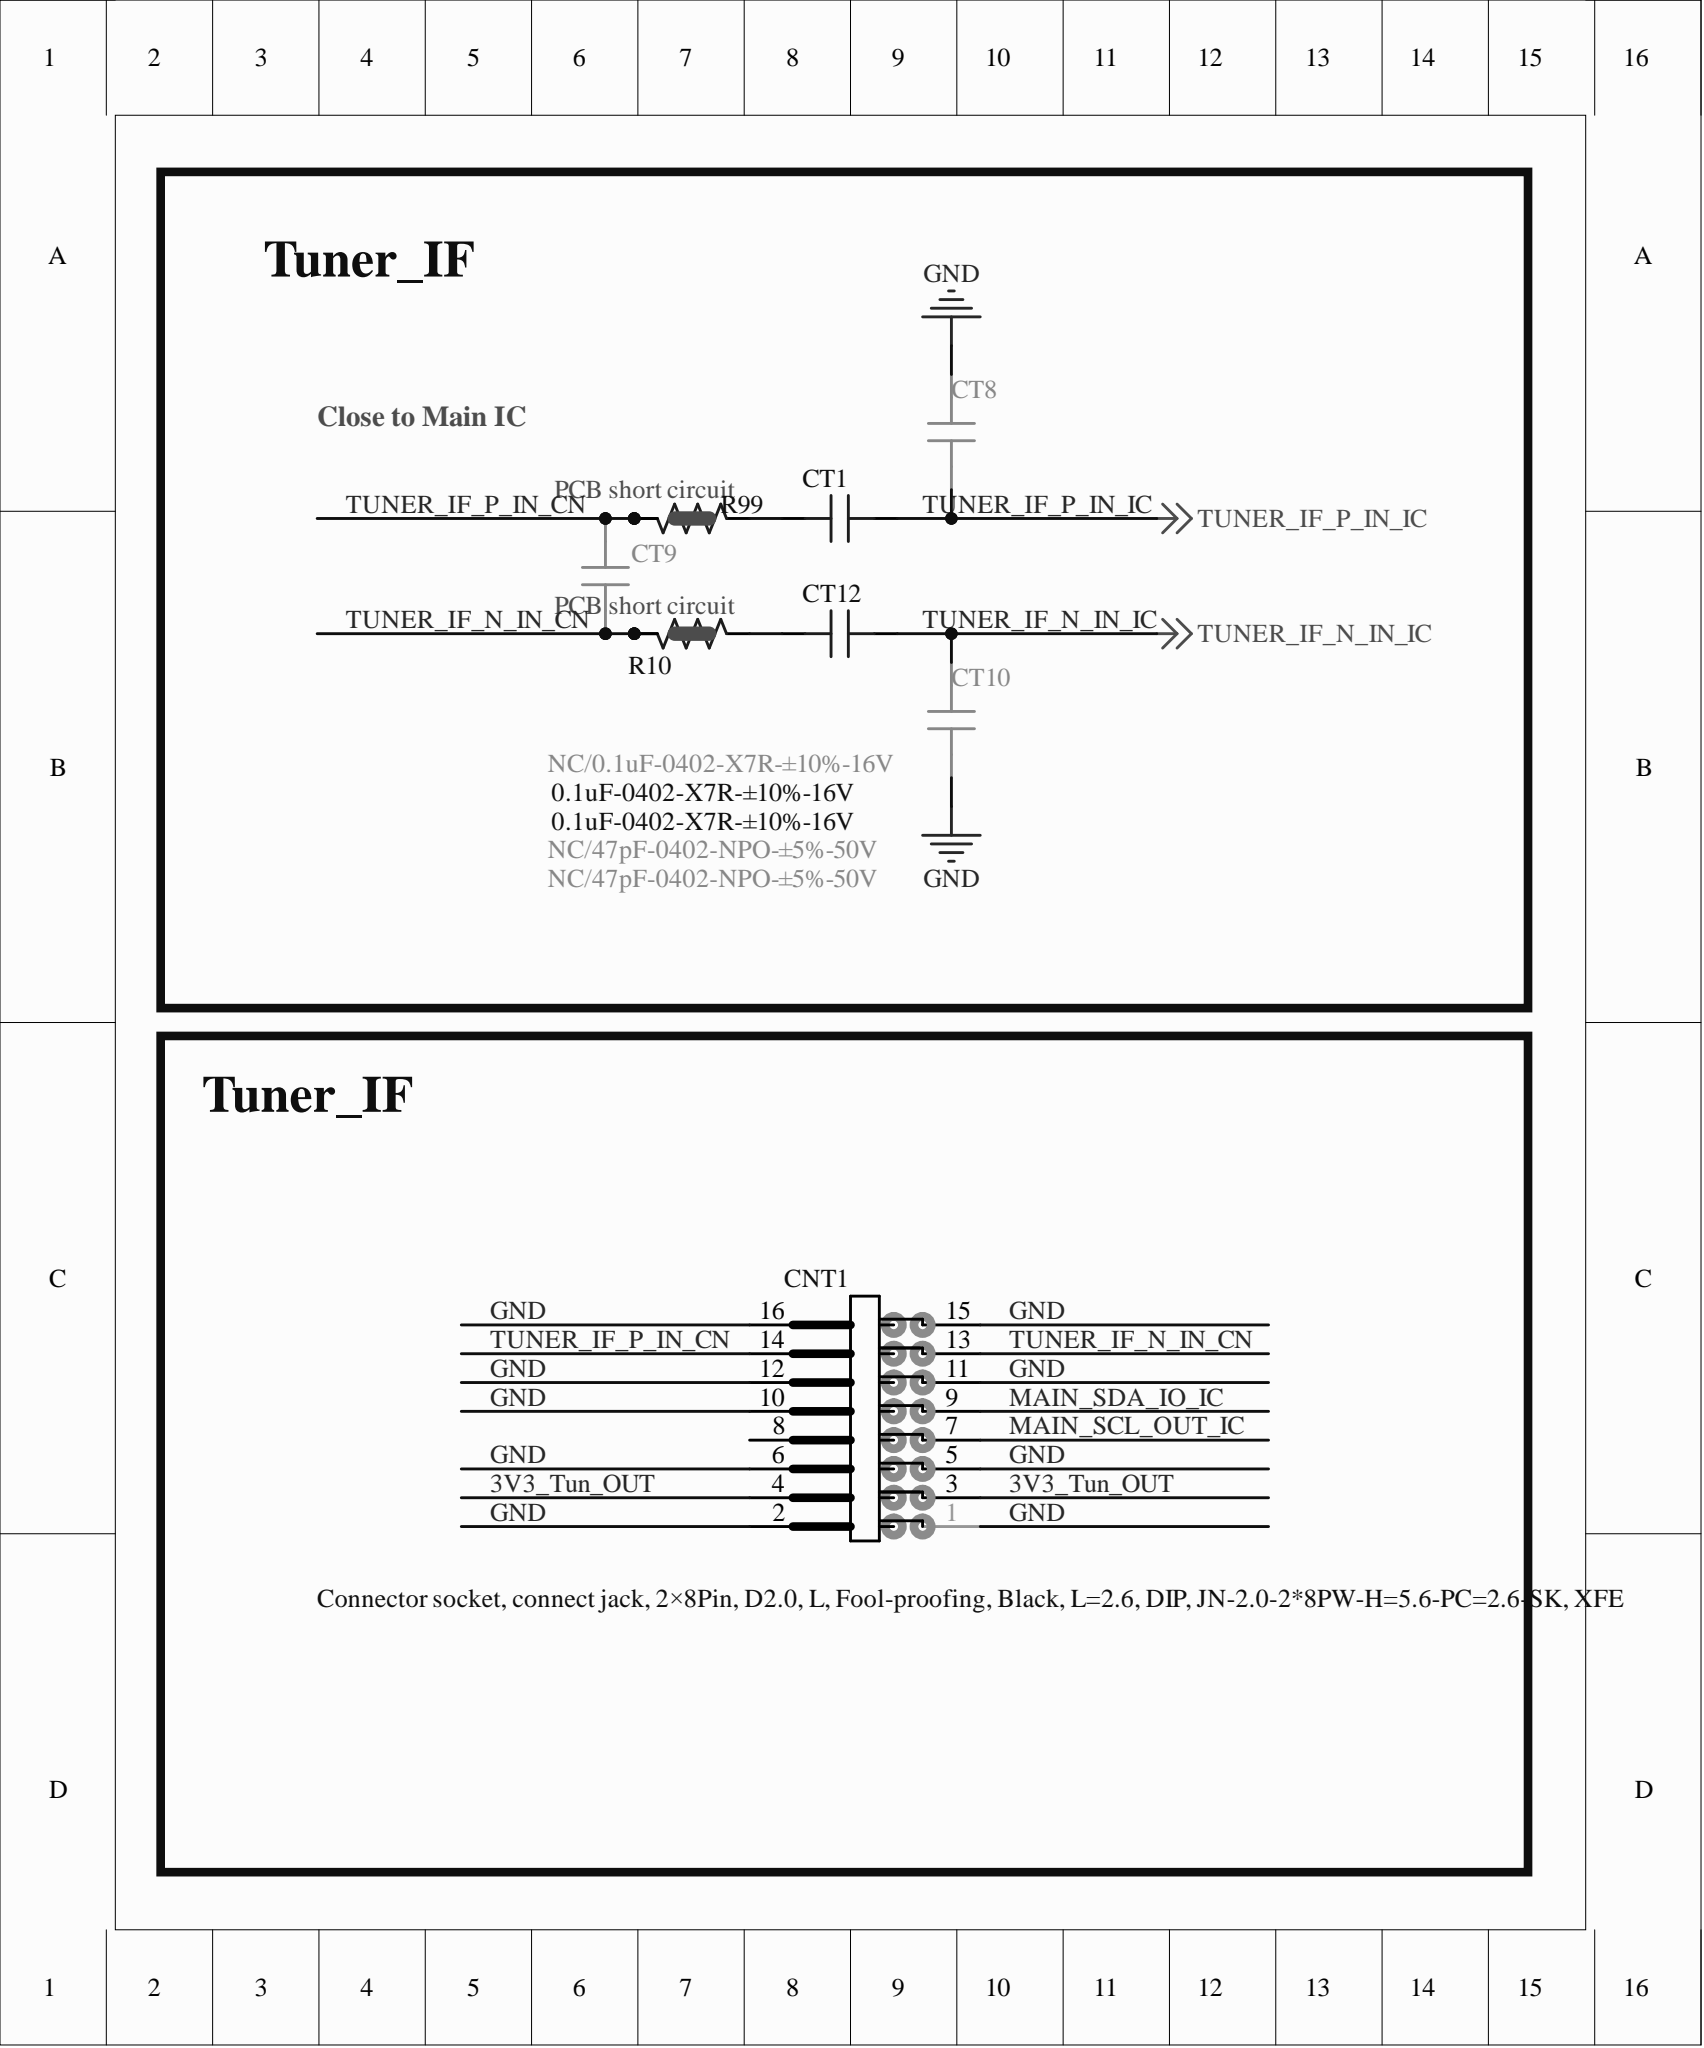Circuit board | Altium Designer | 541 parts | 263 nets | one sheet of the schematic
Parts on this sheet (reference | value | footprint):
CNT1 | Connector socket, connect jack, 2×8Pin, D2.0, L, Fool-proofing, Black, L=2.6, DIP, JN-2.0-2*8PW-H=5.6-PC=2.6-SK, XFE | SIP2*8H/2.0DM-1
CT1 | 0.1uF-0402-X7R-±10%-16V | C0402
CT8 | NC/47pF-0402-NPO-±5%-50V | C0402
CT9 | NC/0.1uF-0402-X7R-±10%-16V | C0402
CT10 | NC/47pF-0402-NPO-±5%-50V | C0402
CT12 | 0.1uF-0402-X7R-±10%-16V | C0402
R10 | NC/0ohm-0402-PCB | R0402SC
R99 | NC/0ohm-0402-PCB | R0402SC
Nets of these parts (net: part-pin ...):
TUNER_IF_P_IN_IC: CT1-1 CT8-2
TUNER_IF_P_IN_CN: CNT1-14 CT9-2 R99-2 R99-3
TUNER_IF_N_IN_IC: CT10-1 CT12-1
TUNER_IF_N_IN_CN: CNT1-13 CT9-1 R10-2 R10-3
NetCT12_2: CT12-2 R10-1
NetCT1_2: CT1-2 R99-1
MAIN_SDA_IO_IC: CNT1-9
MAIN_SCL_OUT_IC: CNT1-7
GND: CNT1-1 CNT1-2 CNT1-5 CNT1-6 CNT1-10 CNT1-11 CNT1-12 CNT1-15 CNT1-16 CT8-1 CT10-2
3V3_Tun_OUT: CNT1-3 CNT1-4